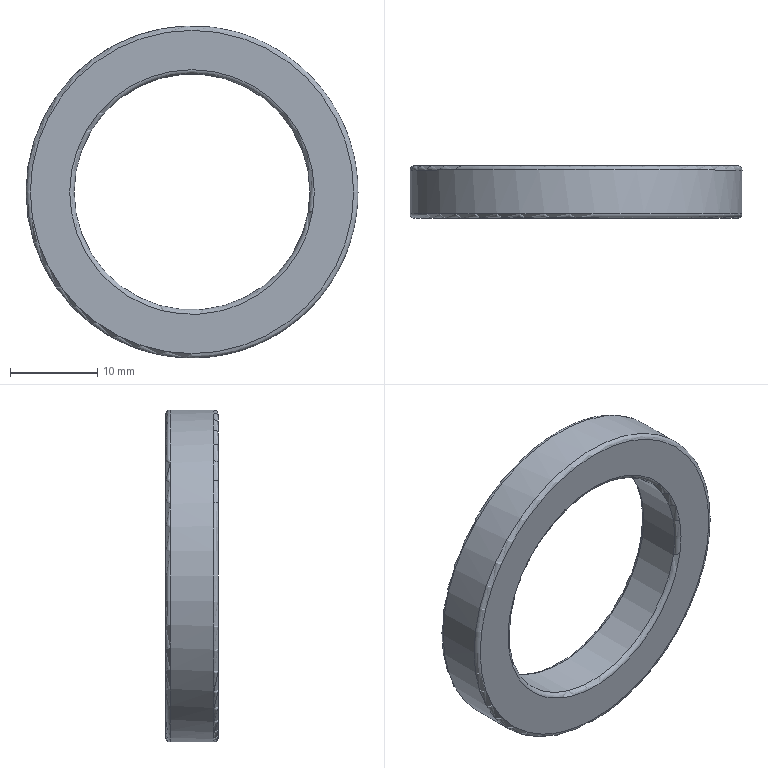Part | STEP file | BK-20_id1226_x_t | 1 solid | 12 faces | box 38 x 6 x 38 mm | volume 1557 mm3 | plane 4 | cylinder 4 | torus 4 | commonest cylinder face diameters 27 x1 29 x1 36 x1 38 x1
STEP:
#1=CARTESIAN_POINT('',(0.,0.,0.));
#2=DIRECTION('',(0.,0.,1.));
#3=DIRECTION('',(1.,0.,0.));
#4=AXIS2_PLACEMENT_3D('',#1,#2,#3);
#5=CARTESIAN_POINT('',(-283.,543.936,-165.5));
#6=VERTEX_POINT('',#5);
#7=CARTESIAN_POINT('',(-268.5,543.936,-165.5));
#8=DIRECTION('',(0.,1.,0.));
#9=DIRECTION('',(-1.,0.,0.));
#10=AXIS2_PLACEMENT_3D('',#7,#8,#9);
#11=CIRCLE('',#10,14.5);
#12=CARTESIAN_POINT('',(-268.5,543.936,-147.5));
#13=DIRECTION('',(0.,-1.,0.));
#14=DIRECTION('',(1.,0.,0.));
#15=AXIS2_PLACEMENT_3D('',#12,#13,#14);
#16=PLANE('',#15);
#17=CARTESIAN_POINT('',(-14.5,-18.));
#18=CARTESIAN_POINT('',(-14.5,7.115));
#19=CARTESIAN_POINT('',(7.25,-5.443));
#20=CARTESIAN_POINT('',(29.,-18.));
#21=CARTESIAN_POINT('',(7.25,-30.557));
#22=CARTESIAN_POINT('',(-14.5,-43.115));
#23=CARTESIAN_POINT('',(-14.5,-18.));
#24=(BOUNDED_CURVE()B_SPLINE_CURVE(2,(#17,#18,#19,#20,#21,#22,#23),.UNSPECIFIED.,.T.,.F.)B_SPLINE_CURVE_WITH_KNOTS((1,2,2,2,2,1),(-2.094,0.,2.094,4.189,6.283,8.378),.UNSPECIFIED.)CURVE()GEOMETRIC_REPRESENTATION_ITEM()RATIONAL_B_SPLINE_CURVE((1.,0.5,1.,0.5,1.,0.5,1.))REPRESENTATION_ITEM(''));
#25=(GEOMETRIC_REPRESENTATION_CONTEXT(2)PARAMETRIC_REPRESENTATION_CONTEXT()REPRESENTATION_CONTEXT('',''));
#26=DEFINITIONAL_REPRESENTATION('',(#24),#25);
#27=PCURVE('',#16,#26);
#28=CARTESIAN_POINT('',(-268.5,569.59,-165.5));
#29=DIRECTION('',(0.,1.,0.));
#30=DIRECTION('',(-1.,0.,0.));
#31=AXIS2_PLACEMENT_3D('',#28,#29,#30);
#32=CYLINDRICAL_SURFACE('',#31,14.5);
#33=CARTESIAN_POINT('',(0.,-25.654));
#34=DIRECTION('',(1.,0.));
#35=VECTOR('',#34,1.);
#36=LINE('',#33,#35);
#37=(GEOMETRIC_REPRESENTATION_CONTEXT(2)PARAMETRIC_REPRESENTATION_CONTEXT()REPRESENTATION_CONTEXT('',''));
#38=DEFINITIONAL_REPRESENTATION('',(#36),#37);
#39=PCURVE('',#32,#38);
#40=SURFACE_CURVE('',#11,(#27,#39),.PCURVE_S1.);
#41=EDGE_CURVE('',#6,#6,#40,.T.);
#42=ORIENTED_EDGE('',*,*,#41,.F.);
#43=EDGE_LOOP('',(#42));
#44=FACE_BOUND('',#43,.T.);
#45=CARTESIAN_POINT('',(-286.5,543.936,-165.5));
#46=VERTEX_POINT('',#45);
#47=CARTESIAN_POINT('',(-268.5,543.936,-165.5));
#48=DIRECTION('',(0.,1.,0.));
#49=DIRECTION('',(-1.,0.,0.));
#50=AXIS2_PLACEMENT_3D('',#47,#48,#49);
#51=CIRCLE('',#50,18.);
#52=CARTESIAN_POINT('',(-18.,-18.));
#53=CARTESIAN_POINT('',(-18.,13.177));
#54=CARTESIAN_POINT('',(9.,-2.412));
#55=CARTESIAN_POINT('',(36.,-18.));
#56=CARTESIAN_POINT('',(9.,-33.588));
#57=CARTESIAN_POINT('',(-18.,-49.177));
#58=CARTESIAN_POINT('',(-18.,-18.));
#59=(BOUNDED_CURVE()B_SPLINE_CURVE(2,(#52,#53,#54,#55,#56,#57,#58),.UNSPECIFIED.,.T.,.F.)B_SPLINE_CURVE_WITH_KNOTS((1,2,2,2,2,1),(-2.094,0.,2.094,4.189,6.283,8.378),.UNSPECIFIED.)CURVE()GEOMETRIC_REPRESENTATION_ITEM()RATIONAL_B_SPLINE_CURVE((1.,0.5,1.,0.5,1.,0.5,1.))REPRESENTATION_ITEM(''));
#60=(GEOMETRIC_REPRESENTATION_CONTEXT(2)PARAMETRIC_REPRESENTATION_CONTEXT()REPRESENTATION_CONTEXT('',''));
#61=DEFINITIONAL_REPRESENTATION('',(#59),#60);
#62=PCURVE('',#16,#61);
#63=CARTESIAN_POINT('',(-268.5,569.59,-165.5));
#64=DIRECTION('',(0.,1.,0.));
#65=DIRECTION('',(-1.,0.,0.));
#66=AXIS2_PLACEMENT_3D('',#63,#64,#65);
#67=CYLINDRICAL_SURFACE('',#66,18.);
#68=CARTESIAN_POINT('',(0.,-25.654));
#69=DIRECTION('',(1.,0.));
#70=VECTOR('',#69,1.);
#71=LINE('',#68,#70);
#72=(GEOMETRIC_REPRESENTATION_CONTEXT(2)PARAMETRIC_REPRESENTATION_CONTEXT()REPRESENTATION_CONTEXT('',''));
#73=DEFINITIONAL_REPRESENTATION('',(#71),#72);
#74=PCURVE('',#67,#73);
#75=SURFACE_CURVE('',#51,(#62,#74),.PCURVE_S1.);
#76=EDGE_CURVE('',#46,#46,#75,.T.);
#77=ORIENTED_EDGE('',*,*,#76,.T.);
#78=EDGE_LOOP('',(#77));
#79=FACE_BOUND('',#78,.T.);
#80=ADVANCED_FACE('',(#44,#79),#16,.F.);
#81=ORIENTED_EDGE('',*,*,#76,.T.);
#82=CARTESIAN_POINT('',(-286.5,548.936,-165.5));
#83=VERTEX_POINT('',#82);
#84=CARTESIAN_POINT('',(-286.5,543.936,-165.5));
#85=CARTESIAN_POINT('',(-286.5,548.936,-165.5));
#86=B_SPLINE_CURVE_WITH_KNOTS('',1,(#84,#85),.UNSPECIFIED.,.F.,.F.,(2,2),(-25.654,-20.654),.PIECEWISE_BEZIER_KNOTS.);
#87=CARTESIAN_POINT('',(6.283,0.));
#88=DIRECTION('',(0.,1.));
#89=VECTOR('',#88,1.);
#90=LINE('',#87,#89);
#91=(GEOMETRIC_REPRESENTATION_CONTEXT(2)PARAMETRIC_REPRESENTATION_CONTEXT()REPRESENTATION_CONTEXT('',''));
#92=DEFINITIONAL_REPRESENTATION('',(#90),#91);
#93=PCURVE('',#67,#92);
#94=CARTESIAN_POINT('',(0.,0.));
#95=DIRECTION('',(0.,1.));
#96=VECTOR('',#95,1.);
#97=LINE('',#94,#96);
#98=(GEOMETRIC_REPRESENTATION_CONTEXT(2)PARAMETRIC_REPRESENTATION_CONTEXT()REPRESENTATION_CONTEXT('',''));
#99=DEFINITIONAL_REPRESENTATION('',(#97),#98);
#100=PCURVE('',#67,#99);
#101=SEAM_CURVE('',#86,(#93,#100),.PCURVE_S1.);
#102=EDGE_CURVE('',#46,#83,#101,.T.);
#103=ORIENTED_EDGE('',*,*,#102,.T.);
#104=CARTESIAN_POINT('',(-268.5,548.936,-165.5));
#105=DIRECTION('',(0.,1.,0.));
#106=DIRECTION('',(-1.,0.,0.));
#107=AXIS2_PLACEMENT_3D('',#104,#105,#106);
#108=CIRCLE('',#107,18.);
#109=CARTESIAN_POINT('',(0.,-20.654));
#110=DIRECTION('',(1.,0.));
#111=VECTOR('',#110,1.);
#112=LINE('',#109,#111);
#113=(GEOMETRIC_REPRESENTATION_CONTEXT(2)PARAMETRIC_REPRESENTATION_CONTEXT()REPRESENTATION_CONTEXT('',''));
#114=DEFINITIONAL_REPRESENTATION('',(#112),#113);
#115=PCURVE('',#67,#114);
#116=CARTESIAN_POINT('',(-268.5,548.936,-146.5));
#117=DIRECTION('',(0.,-1.,0.));
#118=DIRECTION('',(1.,0.,0.));
#119=AXIS2_PLACEMENT_3D('',#116,#117,#118);
#120=PLANE('',#119);
#121=CARTESIAN_POINT('',(-18.,-19.));
#122=CARTESIAN_POINT('',(-18.,12.177));
#123=CARTESIAN_POINT('',(9.,-3.412));
#124=CARTESIAN_POINT('',(36.,-19.));
#125=CARTESIAN_POINT('',(9.,-34.588));
#126=CARTESIAN_POINT('',(-18.,-50.177));
#127=CARTESIAN_POINT('',(-18.,-19.));
#128=(BOUNDED_CURVE()B_SPLINE_CURVE(2,(#121,#122,#123,#124,#125,#126,#127),.UNSPECIFIED.,.T.,.F.)B_SPLINE_CURVE_WITH_KNOTS((1,2,2,2,2,1),(-2.094,0.,2.094,4.189,6.283,8.378),.UNSPECIFIED.)CURVE()GEOMETRIC_REPRESENTATION_ITEM()RATIONAL_B_SPLINE_CURVE((1.,0.5,1.,0.5,1.,0.5,1.))REPRESENTATION_ITEM(''));
#129=(GEOMETRIC_REPRESENTATION_CONTEXT(2)PARAMETRIC_REPRESENTATION_CONTEXT()REPRESENTATION_CONTEXT('',''));
#130=DEFINITIONAL_REPRESENTATION('',(#128),#129);
#131=PCURVE('',#120,#130);
#132=SURFACE_CURVE('',#108,(#115,#131),.PCURVE_S1.);
#133=EDGE_CURVE('',#83,#83,#132,.T.);
#134=ORIENTED_EDGE('',*,*,#133,.F.);
#135=ORIENTED_EDGE('',*,*,#102,.F.);
#136=EDGE_LOOP('',(#81,#103,#134,#135));
#137=FACE_BOUND('',#136,.F.);
#138=ADVANCED_FACE('',(#137),#67,.F.);
#139=ORIENTED_EDGE('',*,*,#41,.T.);
#140=CARTESIAN_POINT('',(-283.,548.936,-165.5));
#141=VERTEX_POINT('',#140);
#142=CARTESIAN_POINT('',(-283.,543.936,-165.5));
#143=CARTESIAN_POINT('',(-283.,548.936,-165.5));
#144=B_SPLINE_CURVE_WITH_KNOTS('',1,(#142,#143),.UNSPECIFIED.,.F.,.F.,(2,2),(-25.654,-20.654),.PIECEWISE_BEZIER_KNOTS.);
#145=CARTESIAN_POINT('',(6.283,0.));
#146=DIRECTION('',(0.,1.));
#147=VECTOR('',#146,1.);
#148=LINE('',#145,#147);
#149=(GEOMETRIC_REPRESENTATION_CONTEXT(2)PARAMETRIC_REPRESENTATION_CONTEXT()REPRESENTATION_CONTEXT('',''));
#150=DEFINITIONAL_REPRESENTATION('',(#148),#149);
#151=PCURVE('',#32,#150);
#152=CARTESIAN_POINT('',(0.,0.));
#153=DIRECTION('',(0.,1.));
#154=VECTOR('',#153,1.);
#155=LINE('',#152,#154);
#156=(GEOMETRIC_REPRESENTATION_CONTEXT(2)PARAMETRIC_REPRESENTATION_CONTEXT()REPRESENTATION_CONTEXT('',''));
#157=DEFINITIONAL_REPRESENTATION('',(#155),#156);
#158=PCURVE('',#32,#157);
#159=SEAM_CURVE('',#144,(#151,#158),.PCURVE_S1.);
#160=EDGE_CURVE('',#6,#141,#159,.T.);
#161=ORIENTED_EDGE('',*,*,#160,.T.);
#162=CARTESIAN_POINT('',(-268.5,548.936,-165.5));
#163=DIRECTION('',(0.,-1.,0.));
#164=DIRECTION('',(-1.,0.,0.));
#165=AXIS2_PLACEMENT_3D('',#162,#163,#164);
#166=CIRCLE('',#165,14.5);
#167=CARTESIAN_POINT('',(6.283,-20.654));
#168=DIRECTION('',(-1.,0.));
#169=VECTOR('',#168,1.);
#170=LINE('',#167,#169);
#171=(GEOMETRIC_REPRESENTATION_CONTEXT(2)PARAMETRIC_REPRESENTATION_CONTEXT()REPRESENTATION_CONTEXT('',''));
#172=DEFINITIONAL_REPRESENTATION('',(#170),#171);
#173=PCURVE('',#32,#172);
#174=CARTESIAN_POINT('',(-268.5,548.936,-151.));
#175=DIRECTION('',(0.,-1.,0.));
#176=DIRECTION('',(1.,0.,0.));
#177=AXIS2_PLACEMENT_3D('',#174,#175,#176);
#178=PLANE('',#177);
#179=CARTESIAN_POINT('',(0.,-14.5));
#180=DIRECTION('',(-1.,0.));
#181=AXIS2_PLACEMENT_2D('',#179,#180);
#182=CIRCLE('',#181,14.5);
#183=(GEOMETRIC_REPRESENTATION_CONTEXT(2)PARAMETRIC_REPRESENTATION_CONTEXT()REPRESENTATION_CONTEXT('',''));
#184=DEFINITIONAL_REPRESENTATION('',(#182),#183);
#185=PCURVE('',#178,#184);
#186=SURFACE_CURVE('',#166,(#173,#185),.PCURVE_S1.);
#187=EDGE_CURVE('',#141,#141,#186,.T.);
#188=ORIENTED_EDGE('',*,*,#187,.T.);
#189=ORIENTED_EDGE('',*,*,#160,.F.);
#190=EDGE_LOOP('',(#139,#161,#188,#189));
#191=FACE_BOUND('',#190,.T.);
#192=ADVANCED_FACE('',(#191),#32,.T.);
#193=CARTESIAN_POINT('',(-250.,548.936,-165.5));
#194=VERTEX_POINT('',#193);
#195=CARTESIAN_POINT('',(-268.5,548.936,-165.5));
#196=DIRECTION('',(0.,-1.,0.));
#197=DIRECTION('',(1.,0.,0.));
#198=AXIS2_PLACEMENT_3D('',#195,#196,#197);
#199=CIRCLE('',#198,18.5);
#200=CARTESIAN_POINT('',(0.,-19.));
#201=DIRECTION('',(1.,0.));
#202=AXIS2_PLACEMENT_2D('',#200,#201);
#203=CIRCLE('',#202,18.5);
#204=(GEOMETRIC_REPRESENTATION_CONTEXT(2)PARAMETRIC_REPRESENTATION_CONTEXT()REPRESENTATION_CONTEXT('',''));
#205=DEFINITIONAL_REPRESENTATION('',(#203),#204);
#206=PCURVE('',#120,#205);
#207=CARTESIAN_POINT('',(-268.5,548.436,-165.5));
#208=DIRECTION('',(0.,-1.,0.));
#209=DIRECTION('',(1.,0.,0.));
#210=AXIS2_PLACEMENT_3D('',#207,#208,#209);
#211=TOROIDAL_SURFACE('',#210,18.5,0.5);
#212=CARTESIAN_POINT('',(0.,4.712));
#213=DIRECTION('',(1.,0.));
#214=VECTOR('',#213,1.);
#215=LINE('',#212,#214);
#216=(GEOMETRIC_REPRESENTATION_CONTEXT(2)PARAMETRIC_REPRESENTATION_CONTEXT()REPRESENTATION_CONTEXT('',''));
#217=DEFINITIONAL_REPRESENTATION('',(#215),#216);
#218=PCURVE('',#211,#217);
#219=SURFACE_CURVE('',#199,(#206,#218),.PCURVE_S1.);
#220=EDGE_CURVE('',#194,#194,#219,.T.);
#221=ORIENTED_EDGE('',*,*,#220,.F.);
#222=EDGE_LOOP('',(#221));
#223=FACE_BOUND('',#222,.T.);
#224=ORIENTED_EDGE('',*,*,#133,.F.);
#225=EDGE_LOOP('',(#224));
#226=FACE_BOUND('',#225,.T.);
#227=ADVANCED_FACE('',(#223,#226),#120,.F.);
#228=CARTESIAN_POINT('',(-254.5,548.936,-165.5));
#229=VERTEX_POINT('',#228);
#230=CARTESIAN_POINT('',(-268.5,548.936,-165.5));
#231=DIRECTION('',(0.,1.,0.));
#232=DIRECTION('',(1.,0.,0.));
#233=AXIS2_PLACEMENT_3D('',#230,#231,#232);
#234=CIRCLE('',#233,14.);
#235=CARTESIAN_POINT('',(14.,-14.5));
#236=CARTESIAN_POINT('',(14.,-38.749));
#237=CARTESIAN_POINT('',(-7.,-26.624));
#238=CARTESIAN_POINT('',(-28.,-14.5));
#239=CARTESIAN_POINT('',(-7.,-2.376));
#240=CARTESIAN_POINT('',(14.,9.749));
#241=CARTESIAN_POINT('',(14.,-14.5));
#242=(BOUNDED_CURVE()B_SPLINE_CURVE(2,(#235,#236,#237,#238,#239,#240,#241),.UNSPECIFIED.,.T.,.F.)B_SPLINE_CURVE_WITH_KNOTS((1,2,2,2,2,1),(-2.094,0.,2.094,4.189,6.283,8.378),.UNSPECIFIED.)CURVE()GEOMETRIC_REPRESENTATION_ITEM()RATIONAL_B_SPLINE_CURVE((1.,0.5,1.,0.5,1.,0.5,1.))REPRESENTATION_ITEM(''));
#243=(GEOMETRIC_REPRESENTATION_CONTEXT(2)PARAMETRIC_REPRESENTATION_CONTEXT()REPRESENTATION_CONTEXT('',''));
#244=DEFINITIONAL_REPRESENTATION('',(#242),#243);
#245=PCURVE('',#178,#244);
#246=CARTESIAN_POINT('',(-268.5,548.436,-165.5));
#247=DIRECTION('',(0.,-1.,0.));
#248=DIRECTION('',(1.,0.,0.));
#249=AXIS2_PLACEMENT_3D('',#246,#247,#248);
#250=TOROIDAL_SURFACE('',#249,14.,0.5);
#251=CARTESIAN_POINT('',(6.283,4.712));
#252=DIRECTION('',(-1.,0.));
#253=VECTOR('',#252,1.);
#254=LINE('',#251,#253);
#255=(GEOMETRIC_REPRESENTATION_CONTEXT(2)PARAMETRIC_REPRESENTATION_CONTEXT()REPRESENTATION_CONTEXT('',''));
#256=DEFINITIONAL_REPRESENTATION('',(#254),#255);
#257=PCURVE('',#250,#256);
#258=SURFACE_CURVE('',#234,(#245,#257),.PCURVE_S1.);
#259=EDGE_CURVE('',#229,#229,#258,.T.);
#260=ORIENTED_EDGE('',*,*,#259,.F.);
#261=EDGE_LOOP('',(#260));
#262=FACE_BOUND('',#261,.T.);
#263=ORIENTED_EDGE('',*,*,#187,.F.);
#264=EDGE_LOOP('',(#263));
#265=FACE_BOUND('',#264,.T.);
#266=ADVANCED_FACE('',(#262,#265),#178,.F.);
#267=CARTESIAN_POINT('',(-249.5,548.436,-165.5));
#268=VERTEX_POINT('',#267);
#269=CARTESIAN_POINT('',(-287.5,548.436,-165.5));
#270=VERTEX_POINT('',#269);
#271=CARTESIAN_POINT('',(-268.5,548.436,-165.5));
#272=DIRECTION('',(0.,-1.,0.));
#273=DIRECTION('',(-1.,0.,0.));
#274=AXIS2_PLACEMENT_3D('',#271,#272,#273);
#275=CIRCLE('',#274,19.);
#276=CARTESIAN_POINT('',(-3.142,6.283));
#277=DIRECTION('',(1.,0.));
#278=VECTOR('',#277,1.);
#279=LINE('',#276,#278);
#280=(GEOMETRIC_REPRESENTATION_CONTEXT(2)PARAMETRIC_REPRESENTATION_CONTEXT()REPRESENTATION_CONTEXT('',''));
#281=DEFINITIONAL_REPRESENTATION('',(#279),#280);
#282=PCURVE('',#211,#281);
#283=CARTESIAN_POINT('',(-268.5,569.59,-165.5));
#284=DIRECTION('',(0.,1.,0.));
#285=DIRECTION('',(-1.,0.,0.));
#286=AXIS2_PLACEMENT_3D('',#283,#284,#285);
#287=CYLINDRICAL_SURFACE('',#286,19.);
#288=CARTESIAN_POINT('',(6.283,-21.154));
#289=DIRECTION('',(-1.,0.));
#290=VECTOR('',#289,1.);
#291=LINE('',#288,#290);
#292=(GEOMETRIC_REPRESENTATION_CONTEXT(2)PARAMETRIC_REPRESENTATION_CONTEXT()REPRESENTATION_CONTEXT('',''));
#293=DEFINITIONAL_REPRESENTATION('',(#291),#292);
#294=PCURVE('',#287,#293);
#295=SURFACE_CURVE('',#275,(#282,#294),.PCURVE_S1.);
#296=EDGE_CURVE('',#268,#270,#295,.T.);
#297=ORIENTED_EDGE('',*,*,#296,.F.);
#298=CARTESIAN_POINT('',(-250.,548.936,-165.5));
#299=CARTESIAN_POINT('',(-249.866,548.936,-165.5));
#300=CARTESIAN_POINT('',(-249.736,548.893,-165.5));
#301=CARTESIAN_POINT('',(-249.624,548.812,-165.5));
#302=CARTESIAN_POINT('',(-249.543,548.699,-165.5));
#303=CARTESIAN_POINT('',(-249.5,548.569,-165.5));
#304=CARTESIAN_POINT('',(-249.5,548.436,-165.5));
#305=(BOUNDED_CURVE()B_SPLINE_CURVE(6,(#298,#299,#300,#301,#302,#303,#304),.UNSPECIFIED.,.F.,.F.)B_SPLINE_CURVE_WITH_KNOTS((7,7),(-1.571,0.),.PIECEWISE_BEZIER_KNOTS.)CURVE()GEOMETRIC_REPRESENTATION_ITEM()RATIONAL_B_SPLINE_CURVE((1.031,1.01,0.9979,0.994,0.9979,1.01,1.031))REPRESENTATION_ITEM(''));
#306=CARTESIAN_POINT('',(0.,6.283));
#307=DIRECTION('',(0.,1.));
#308=VECTOR('',#307,1.);
#309=LINE('',#306,#308);
#310=(GEOMETRIC_REPRESENTATION_CONTEXT(2)PARAMETRIC_REPRESENTATION_CONTEXT()REPRESENTATION_CONTEXT('',''));
#311=DEFINITIONAL_REPRESENTATION('',(#309),#310);
#312=PCURVE('',#211,#311);
#313=CARTESIAN_POINT('',(6.283,6.283));
#314=DIRECTION('',(0.,1.));
#315=VECTOR('',#314,1.);
#316=LINE('',#313,#315);
#317=(GEOMETRIC_REPRESENTATION_CONTEXT(2)PARAMETRIC_REPRESENTATION_CONTEXT()REPRESENTATION_CONTEXT('',''));
#318=DEFINITIONAL_REPRESENTATION('',(#316),#317);
#319=PCURVE('',#211,#318);
#320=SEAM_CURVE('',#305,(#312,#319),.PCURVE_S1.);
#321=EDGE_CURVE('',#194,#268,#320,.T.);
#322=ORIENTED_EDGE('',*,*,#321,.F.);
#323=ORIENTED_EDGE('',*,*,#220,.T.);
#324=ORIENTED_EDGE('',*,*,#321,.T.);
#325=CARTESIAN_POINT('',(-268.5,548.436,-165.5));
#326=DIRECTION('',(0.,-1.,0.));
#327=DIRECTION('',(-1.,0.,0.));
#328=AXIS2_PLACEMENT_3D('',#325,#326,#327);
#329=CIRCLE('',#328,19.);
#330=CARTESIAN_POINT('',(3.142,6.283));
#331=DIRECTION('',(1.,0.));
#332=VECTOR('',#331,1.);
#333=LINE('',#330,#332);
#334=(GEOMETRIC_REPRESENTATION_CONTEXT(2)PARAMETRIC_REPRESENTATION_CONTEXT()REPRESENTATION_CONTEXT('',''));
#335=DEFINITIONAL_REPRESENTATION('',(#333),#334);
#336=PCURVE('',#211,#335);
#337=CARTESIAN_POINT('',(6.283,-21.154));
#338=DIRECTION('',(-1.,0.));
#339=VECTOR('',#338,1.);
#340=LINE('',#337,#339);
#341=(GEOMETRIC_REPRESENTATION_CONTEXT(2)PARAMETRIC_REPRESENTATION_CONTEXT()REPRESENTATION_CONTEXT('',''));
#342=DEFINITIONAL_REPRESENTATION('',(#340),#341);
#343=PCURVE('',#287,#342);
#344=SURFACE_CURVE('',#329,(#336,#343),.PCURVE_S1.);
#345=EDGE_CURVE('',#270,#268,#344,.T.);
#346=ORIENTED_EDGE('',*,*,#345,.F.);
#347=EDGE_LOOP('',(#297,#322,#323,#324,#346));
#348=FACE_BOUND('',#347,.T.);
#349=ADVANCED_FACE('',(#348),#211,.T.);
#350=CARTESIAN_POINT('',(-282.,548.436,-165.5));
#351=VERTEX_POINT('',#350);
#352=CARTESIAN_POINT('',(-255.,548.436,-165.5));
#353=VERTEX_POINT('',#352);
#354=CARTESIAN_POINT('',(-268.5,548.436,-165.5));
#355=DIRECTION('',(0.,-1.,0.));
#356=DIRECTION('',(-1.,0.,0.));
#357=AXIS2_PLACEMENT_3D('',#354,#355,#356);
#358=CIRCLE('',#357,13.5);
#359=CARTESIAN_POINT('',(3.142,3.142));
#360=DIRECTION('',(1.,0.));
#361=VECTOR('',#360,1.);
#362=LINE('',#359,#361);
#363=(GEOMETRIC_REPRESENTATION_CONTEXT(2)PARAMETRIC_REPRESENTATION_CONTEXT()REPRESENTATION_CONTEXT('',''));
#364=DEFINITIONAL_REPRESENTATION('',(#362),#363);
#365=PCURVE('',#250,#364);
#366=CARTESIAN_POINT('',(-268.5,569.59,-165.5));
#367=DIRECTION('',(0.,1.,0.));
#368=DIRECTION('',(-1.,0.,0.));
#369=AXIS2_PLACEMENT_3D('',#366,#367,#368);
#370=CYLINDRICAL_SURFACE('',#369,13.5);
#371=CARTESIAN_POINT('',(6.283,-21.154));
#372=DIRECTION('',(-1.,0.));
#373=VECTOR('',#372,1.);
#374=LINE('',#371,#373);
#375=(GEOMETRIC_REPRESENTATION_CONTEXT(2)PARAMETRIC_REPRESENTATION_CONTEXT()REPRESENTATION_CONTEXT('',''));
#376=DEFINITIONAL_REPRESENTATION('',(#374),#375);
#377=PCURVE('',#370,#376);
#378=SURFACE_CURVE('',#358,(#365,#377),.PCURVE_S1.);
#379=EDGE_CURVE('',#351,#353,#378,.T.);
#380=ORIENTED_EDGE('',*,*,#379,.T.);
#381=CARTESIAN_POINT('',(-255.,548.436,-165.5));
#382=CARTESIAN_POINT('',(-255.,548.569,-165.5));
#383=CARTESIAN_POINT('',(-254.957,548.699,-165.5));
#384=CARTESIAN_POINT('',(-254.876,548.812,-165.5));
#385=CARTESIAN_POINT('',(-254.764,548.893,-165.5));
#386=CARTESIAN_POINT('',(-254.634,548.936,-165.5));
#387=CARTESIAN_POINT('',(-254.5,548.936,-165.5));
#388=(BOUNDED_CURVE()B_SPLINE_CURVE(6,(#381,#382,#383,#384,#385,#386,#387),.UNSPECIFIED.,.F.,.F.)B_SPLINE_CURVE_WITH_KNOTS((7,7),(3.142,4.712),.PIECEWISE_BEZIER_KNOTS.)CURVE()GEOMETRIC_REPRESENTATION_ITEM()RATIONAL_B_SPLINE_CURVE((1.031,1.01,0.9979,0.994,0.9979,1.01,1.031))REPRESENTATION_ITEM(''));
#389=CARTESIAN_POINT('',(6.283,0.));
#390=DIRECTION('',(0.,1.));
#391=VECTOR('',#390,1.);
#392=LINE('',#389,#391);
#393=(GEOMETRIC_REPRESENTATION_CONTEXT(2)PARAMETRIC_REPRESENTATION_CONTEXT()REPRESENTATION_CONTEXT('',''));
#394=DEFINITIONAL_REPRESENTATION('',(#392),#393);
#395=PCURVE('',#250,#394);
#396=CARTESIAN_POINT('',(0.,0.));
#397=DIRECTION('',(0.,1.));
#398=VECTOR('',#397,1.);
#399=LINE('',#396,#398);
#400=(GEOMETRIC_REPRESENTATION_CONTEXT(2)PARAMETRIC_REPRESENTATION_CONTEXT()REPRESENTATION_CONTEXT('',''));
#401=DEFINITIONAL_REPRESENTATION('',(#399),#400);
#402=PCURVE('',#250,#401);
#403=SEAM_CURVE('',#388,(#395,#402),.PCURVE_S1.);
#404=EDGE_CURVE('',#353,#229,#403,.T.);
#405=ORIENTED_EDGE('',*,*,#404,.T.);
#406=ORIENTED_EDGE('',*,*,#259,.T.);
#407=ORIENTED_EDGE('',*,*,#404,.F.);
#408=CARTESIAN_POINT('',(-268.5,548.436,-165.5));
#409=DIRECTION('',(0.,-1.,0.));
#410=DIRECTION('',(-1.,0.,0.));
#411=AXIS2_PLACEMENT_3D('',#408,#409,#410);
#412=CIRCLE('',#411,13.5);
#413=CARTESIAN_POINT('',(-3.142,3.142));
#414=DIRECTION('',(1.,0.));
#415=VECTOR('',#414,1.);
#416=LINE('',#413,#415);
#417=(GEOMETRIC_REPRESENTATION_CONTEXT(2)PARAMETRIC_REPRESENTATION_CONTEXT()REPRESENTATION_CONTEXT('',''));
#418=DEFINITIONAL_REPRESENTATION('',(#416),#417);
#419=PCURVE('',#250,#418);
#420=CARTESIAN_POINT('',(12.566,-21.154));
#421=DIRECTION('',(-1.,0.));
#422=VECTOR('',#421,1.);
#423=LINE('',#420,#422);
#424=(GEOMETRIC_REPRESENTATION_CONTEXT(2)PARAMETRIC_REPRESENTATION_CONTEXT()REPRESENTATION_CONTEXT('',''));
#425=DEFINITIONAL_REPRESENTATION('',(#423),#424);
#426=PCURVE('',#370,#425);
#427=SURFACE_CURVE('',#412,(#419,#426),.PCURVE_S1.);
#428=EDGE_CURVE('',#353,#351,#427,.T.);
#429=ORIENTED_EDGE('',*,*,#428,.T.);
#430=EDGE_LOOP('',(#380,#405,#406,#407,#429));
#431=FACE_BOUND('',#430,.T.);
#432=ADVANCED_FACE('',(#431),#250,.T.);
#433=ORIENTED_EDGE('',*,*,#345,.T.);
#434=ORIENTED_EDGE('',*,*,#296,.T.);
#435=CARTESIAN_POINT('',(-287.5,543.436,-165.5));
#436=VERTEX_POINT('',#435);
#437=CARTESIAN_POINT('',(-287.5,543.436,-165.5));
#438=CARTESIAN_POINT('',(-287.5,548.436,-165.5));
#439=B_SPLINE_CURVE_WITH_KNOTS('',1,(#437,#438),.UNSPECIFIED.,.F.,.F.,(2,2),(-26.154,-21.154),.PIECEWISE_BEZIER_KNOTS.);
#440=CARTESIAN_POINT('',(0.,0.));
#441=DIRECTION('',(0.,1.));
#442=VECTOR('',#441,1.);
#443=LINE('',#440,#442);
#444=(GEOMETRIC_REPRESENTATION_CONTEXT(2)PARAMETRIC_REPRESENTATION_CONTEXT()REPRESENTATION_CONTEXT('',''));
#445=DEFINITIONAL_REPRESENTATION('',(#443),#444);
#446=PCURVE('',#287,#445);
#447=CARTESIAN_POINT('',(6.283,0.));
#448=DIRECTION('',(0.,1.));
#449=VECTOR('',#448,1.);
#450=LINE('',#447,#449);
#451=(GEOMETRIC_REPRESENTATION_CONTEXT(2)PARAMETRIC_REPRESENTATION_CONTEXT()REPRESENTATION_CONTEXT('',''));
#452=DEFINITIONAL_REPRESENTATION('',(#450),#451);
#453=PCURVE('',#287,#452);
#454=SEAM_CURVE('',#439,(#446,#453),.PCURVE_S1.);
#455=EDGE_CURVE('',#436,#270,#454,.T.);
#456=ORIENTED_EDGE('',*,*,#455,.F.);
#457=CARTESIAN_POINT('',(-268.5,543.436,-165.5));
#458=DIRECTION('',(0.,-1.,0.));
#459=DIRECTION('',(-1.,0.,0.));
#460=AXIS2_PLACEMENT_3D('',#457,#458,#459);
#461=CIRCLE('',#460,19.);
#462=CARTESIAN_POINT('',(6.283,-26.154));
#463=DIRECTION('',(-1.,0.));
#464=VECTOR('',#463,1.);
#465=LINE('',#462,#464);
#466=(GEOMETRIC_REPRESENTATION_CONTEXT(2)PARAMETRIC_REPRESENTATION_CONTEXT()REPRESENTATION_CONTEXT('',''));
#467=DEFINITIONAL_REPRESENTATION('',(#465),#466);
#468=PCURVE('',#287,#467);
#469=CARTESIAN_POINT('',(-268.5,543.436,-165.5));
#470=DIRECTION('',(0.,1.,0.));
#471=DIRECTION('',(-1.,0.,0.));
#472=AXIS2_PLACEMENT_3D('',#469,#470,#471);
#473=TOROIDAL_SURFACE('',#472,18.5,0.5);
#474=CARTESIAN_POINT('',(6.283,6.283));
#475=DIRECTION('',(-1.,0.));
#476=VECTOR('',#475,1.);
#477=LINE('',#474,#476);
#478=(GEOMETRIC_REPRESENTATION_CONTEXT(2)PARAMETRIC_REPRESENTATION_CONTEXT()REPRESENTATION_CONTEXT('',''));
#479=DEFINITIONAL_REPRESENTATION('',(#477),#478);
#480=PCURVE('',#473,#479);
#481=SURFACE_CURVE('',#461,(#468,#480),.PCURVE_S1.);
#482=EDGE_CURVE('',#436,#436,#481,.T.);
#483=ORIENTED_EDGE('',*,*,#482,.F.);
#484=ORIENTED_EDGE('',*,*,#455,.T.);
#485=EDGE_LOOP('',(#433,#434,#456,#483,#484));
#486=FACE_BOUND('',#485,.T.);
#487=ADVANCED_FACE('',(#486),#287,.T.);
#488=ORIENTED_EDGE('',*,*,#428,.T.);
#489=ORIENTED_EDGE('',*,*,#379,.T.);
#490=CARTESIAN_POINT('',(-255.,543.436,-165.5));
#491=VERTEX_POINT('',#490);
#492=CARTESIAN_POINT('',(-255.,543.436,-165.5));
#493=CARTESIAN_POINT('',(-255.,548.436,-165.5));
#494=B_SPLINE_CURVE_WITH_KNOTS('',1,(#492,#493),.UNSPECIFIED.,.F.,.F.,(2,2),(-26.154,-21.154),.PIECEWISE_BEZIER_KNOTS.);
#495=CARTESIAN_POINT('',(3.142,0.));
#496=DIRECTION('',(0.,1.));
#497=VECTOR('',#496,1.);
#498=LINE('',#495,#497);
#499=(GEOMETRIC_REPRESENTATION_CONTEXT(2)PARAMETRIC_REPRESENTATION_CONTEXT()REPRESENTATION_CONTEXT('',''));
#500=DEFINITIONAL_REPRESENTATION('',(#498),#499);
#501=PCURVE('',#370,#500);
#502=CARTESIAN_POINT('',(9.425,0.));
#503=DIRECTION('',(0.,1.));
#504=VECTOR('',#503,1.);
#505=LINE('',#502,#504);
#506=(GEOMETRIC_REPRESENTATION_CONTEXT(2)PARAMETRIC_REPRESENTATION_CONTEXT()REPRESENTATION_CONTEXT('',''));
#507=DEFINITIONAL_REPRESENTATION('',(#505),#506);
#508=PCURVE('',#370,#507);
#509=SEAM_CURVE('',#494,(#501,#508),.PCURVE_S1.);
#510=EDGE_CURVE('',#491,#353,#509,.T.);
#511=ORIENTED_EDGE('',*,*,#510,.F.);
#512=CARTESIAN_POINT('',(-268.5,543.436,-165.5));
#513=DIRECTION('',(0.,1.,0.));
#514=DIRECTION('',(1.,0.,0.));
#515=AXIS2_PLACEMENT_3D('',#512,#513,#514);
#516=CIRCLE('',#515,13.5);
#517=CARTESIAN_POINT('',(3.142,-26.154));
#518=DIRECTION('',(1.,0.));
#519=VECTOR('',#518,1.);
#520=LINE('',#517,#519);
#521=(GEOMETRIC_REPRESENTATION_CONTEXT(2)PARAMETRIC_REPRESENTATION_CONTEXT()REPRESENTATION_CONTEXT('',''));
#522=DEFINITIONAL_REPRESENTATION('',(#520),#521);
#523=PCURVE('',#370,#522);
#524=CARTESIAN_POINT('',(-268.5,543.436,-165.5));
#525=DIRECTION('',(0.,1.,0.));
#526=DIRECTION('',(0.,0.,-1.));
#527=AXIS2_PLACEMENT_3D('',#524,#525,#526);
#528=TOROIDAL_SURFACE('',#527,14.,0.5);
#529=CARTESIAN_POINT('',(4.712,3.142));
#530=DIRECTION('',(1.,0.));
#531=VECTOR('',#530,1.);
#532=LINE('',#529,#531);
#533=(GEOMETRIC_REPRESENTATION_CONTEXT(2)PARAMETRIC_REPRESENTATION_CONTEXT()REPRESENTATION_CONTEXT('',''));
#534=DEFINITIONAL_REPRESENTATION('',(#532),#533);
#535=PCURVE('',#528,#534);
#536=SURFACE_CURVE('',#516,(#523,#535),.PCURVE_S1.);
#537=EDGE_CURVE('',#491,#491,#536,.T.);
#538=ORIENTED_EDGE('',*,*,#537,.T.);
#539=ORIENTED_EDGE('',*,*,#510,.T.);
#540=EDGE_LOOP('',(#488,#489,#511,#538,#539));
#541=FACE_BOUND('',#540,.F.);
#542=ADVANCED_FACE('',(#541),#370,.F.);
#543=ORIENTED_EDGE('',*,*,#482,.T.);
#544=CARTESIAN_POINT('',(-287.,542.936,-165.5));
#545=VERTEX_POINT('',#544);
#546=CARTESIAN_POINT('',(-287.,542.936,-165.5));
#547=CARTESIAN_POINT('',(-287.134,542.936,-165.5));
#548=CARTESIAN_POINT('',(-287.264,542.978,-165.5));
#549=CARTESIAN_POINT('',(-287.376,543.06,-165.5));
#550=CARTESIAN_POINT('',(-287.457,543.172,-165.5));
#551=CARTESIAN_POINT('',(-287.5,543.302,-165.5));
#552=CARTESIAN_POINT('',(-287.5,543.436,-165.5));
#553=(BOUNDED_CURVE()B_SPLINE_CURVE(6,(#546,#547,#548,#549,#550,#551,#552),.UNSPECIFIED.,.F.,.F.)B_SPLINE_CURVE_WITH_KNOTS((7,7),(-1.571,0.),.PIECEWISE_BEZIER_KNOTS.)CURVE()GEOMETRIC_REPRESENTATION_ITEM()RATIONAL_B_SPLINE_CURVE((1.031,1.01,0.9979,0.994,0.9979,1.01,1.031))REPRESENTATION_ITEM(''));
#554=CARTESIAN_POINT('',(0.,6.283));
#555=DIRECTION('',(0.,1.));
#556=VECTOR('',#555,1.);
#557=LINE('',#554,#556);
#558=(GEOMETRIC_REPRESENTATION_CONTEXT(2)PARAMETRIC_REPRESENTATION_CONTEXT()REPRESENTATION_CONTEXT('',''));
#559=DEFINITIONAL_REPRESENTATION('',(#557),#558);
#560=PCURVE('',#473,#559);
#561=CARTESIAN_POINT('',(6.283,6.283));
#562=DIRECTION('',(0.,1.));
#563=VECTOR('',#562,1.);
#564=LINE('',#561,#563);
#565=(GEOMETRIC_REPRESENTATION_CONTEXT(2)PARAMETRIC_REPRESENTATION_CONTEXT()REPRESENTATION_CONTEXT('',''));
#566=DEFINITIONAL_REPRESENTATION('',(#564),#565);
#567=PCURVE('',#473,#566);
#568=SEAM_CURVE('',#553,(#560,#567),.PCURVE_S1.);
#569=EDGE_CURVE('',#545,#436,#568,.T.);
#570=ORIENTED_EDGE('',*,*,#569,.F.);
#571=CARTESIAN_POINT('',(-268.5,542.936,-165.5));
#572=DIRECTION('',(0.,1.,0.));
#573=DIRECTION('',(-1.,0.,0.));
#574=AXIS2_PLACEMENT_3D('',#571,#572,#573);
#575=CIRCLE('',#574,18.5);
#576=CARTESIAN_POINT('',(0.,4.712));
#577=DIRECTION('',(1.,0.));
#578=VECTOR('',#577,1.);
#579=LINE('',#576,#578);
#580=(GEOMETRIC_REPRESENTATION_CONTEXT(2)PARAMETRIC_REPRESENTATION_CONTEXT()REPRESENTATION_CONTEXT('',''));
#581=DEFINITIONAL_REPRESENTATION('',(#579),#580);
#582=PCURVE('',#473,#581);
#583=CARTESIAN_POINT('',(-268.5,542.936,-146.5));
#584=DIRECTION('',(0.,1.,0.));
#585=DIRECTION('',(-1.,0.,0.));
#586=AXIS2_PLACEMENT_3D('',#583,#584,#585);
#587=PLANE('',#586);
#588=CARTESIAN_POINT('',(0.,-19.));
#589=DIRECTION('',(1.,0.));
#590=AXIS2_PLACEMENT_2D('',#588,#589);
#591=CIRCLE('',#590,18.5);
#592=(GEOMETRIC_REPRESENTATION_CONTEXT(2)PARAMETRIC_REPRESENTATION_CONTEXT()REPRESENTATION_CONTEXT('',''));
#593=DEFINITIONAL_REPRESENTATION('',(#591),#592);
#594=PCURVE('',#587,#593);
#595=SURFACE_CURVE('',#575,(#582,#594),.PCURVE_S1.);
#596=EDGE_CURVE('',#545,#545,#595,.T.);
#597=ORIENTED_EDGE('',*,*,#596,.T.);
#598=ORIENTED_EDGE('',*,*,#569,.T.);
#599=EDGE_LOOP('',(#543,#570,#597,#598));
#600=FACE_BOUND('',#599,.T.);
#601=ADVANCED_FACE('',(#600),#473,.T.);
#602=ORIENTED_EDGE('',*,*,#537,.T.);
#603=CARTESIAN_POINT('',(-254.5,542.936,-165.5));
#604=VERTEX_POINT('',#603);
#605=CARTESIAN_POINT('',(-255.,543.436,-165.5));
#606=CARTESIAN_POINT('',(-255.,543.302,-165.5));
#607=CARTESIAN_POINT('',(-254.957,543.172,-165.5));
#608=CARTESIAN_POINT('',(-254.876,543.06,-165.5));
#609=CARTESIAN_POINT('',(-254.764,542.978,-165.5));
#610=CARTESIAN_POINT('',(-254.634,542.936,-165.5));
#611=CARTESIAN_POINT('',(-254.5,542.936,-165.5));
#612=(BOUNDED_CURVE()B_SPLINE_CURVE(6,(#605,#606,#607,#608,#609,#610,#611),.UNSPECIFIED.,.F.,.F.)B_SPLINE_CURVE_WITH_KNOTS((7,7),(3.142,4.712),.PIECEWISE_BEZIER_KNOTS.)CURVE()GEOMETRIC_REPRESENTATION_ITEM()RATIONAL_B_SPLINE_CURVE((1.031,1.01,0.9979,0.994,0.9979,1.01,1.031))REPRESENTATION_ITEM(''));
#613=CARTESIAN_POINT('',(10.996,0.));
#614=DIRECTION('',(0.,1.));
#615=VECTOR('',#614,1.);
#616=LINE('',#613,#615);
#617=(GEOMETRIC_REPRESENTATION_CONTEXT(2)PARAMETRIC_REPRESENTATION_CONTEXT()REPRESENTATION_CONTEXT('',''));
#618=DEFINITIONAL_REPRESENTATION('',(#616),#617);
#619=PCURVE('',#528,#618);
#620=CARTESIAN_POINT('',(4.712,0.));
#621=DIRECTION('',(0.,1.));
#622=VECTOR('',#621,1.);
#623=LINE('',#620,#622);
#624=(GEOMETRIC_REPRESENTATION_CONTEXT(2)PARAMETRIC_REPRESENTATION_CONTEXT()REPRESENTATION_CONTEXT('',''));
#625=DEFINITIONAL_REPRESENTATION('',(#623),#624);
#626=PCURVE('',#528,#625);
#627=SEAM_CURVE('',#612,(#619,#626),.PCURVE_S1.);
#628=EDGE_CURVE('',#491,#604,#627,.T.);
#629=ORIENTED_EDGE('',*,*,#628,.T.);
#630=CARTESIAN_POINT('',(-282.5,542.936,-165.5));
#631=VERTEX_POINT('',#630);
#632=CARTESIAN_POINT('',(-268.5,542.936,-165.5));
#633=DIRECTION('',(0.,-1.,0.));
#634=DIRECTION('',(0.,0.,-1.));
#635=AXIS2_PLACEMENT_3D('',#632,#633,#634);
#636=CIRCLE('',#635,14.);
#637=CARTESIAN_POINT('',(12.566,4.712));
#638=DIRECTION('',(-1.,0.));
#639=VECTOR('',#638,1.);
#640=LINE('',#637,#639);
#641=(GEOMETRIC_REPRESENTATION_CONTEXT(2)PARAMETRIC_REPRESENTATION_CONTEXT()REPRESENTATION_CONTEXT('',''));
#642=DEFINITIONAL_REPRESENTATION('',(#640),#641);
#643=PCURVE('',#528,#642);
#644=CARTESIAN_POINT('',(0.,-33.));
#645=CARTESIAN_POINT('',(-24.249,-33.));
#646=CARTESIAN_POINT('',(-12.124,-12.));
#647=CARTESIAN_POINT('',(0.,9.));
#648=CARTESIAN_POINT('',(12.124,-12.));
#649=CARTESIAN_POINT('',(24.249,-33.));
#650=CARTESIAN_POINT('',(0.,-33.));
#651=(BOUNDED_CURVE()B_SPLINE_CURVE(2,(#644,#645,#646,#647,#648,#649,#650),.UNSPECIFIED.,.T.,.F.)B_SPLINE_CURVE_WITH_KNOTS((1,2,2,2,2,1),(-2.094,0.,2.094,4.189,6.283,8.378),.UNSPECIFIED.)CURVE()GEOMETRIC_REPRESENTATION_ITEM()RATIONAL_B_SPLINE_CURVE((1.,0.5,1.,0.5,1.,0.5,1.))REPRESENTATION_ITEM(''));
#652=(GEOMETRIC_REPRESENTATION_CONTEXT(2)PARAMETRIC_REPRESENTATION_CONTEXT()REPRESENTATION_CONTEXT('',''));
#653=DEFINITIONAL_REPRESENTATION('',(#651),#652);
#654=PCURVE('',#587,#653);
#655=SURFACE_CURVE('',#636,(#643,#654),.PCURVE_S1.);
#656=EDGE_CURVE('',#604,#631,#655,.T.);
#657=ORIENTED_EDGE('',*,*,#656,.T.);
#658=CARTESIAN_POINT('',(-282.5,542.936,-165.5));
#659=CARTESIAN_POINT('',(-282.5,542.936,-165.831));
#660=CARTESIAN_POINT('',(-282.488,542.936,-166.162));
#661=CARTESIAN_POINT('',(-282.453,542.936,-166.658));
#662=CARTESIAN_POINT('',(-282.431,542.936,-166.905));
#663=CARTESIAN_POINT('',(-282.403,542.936,-167.152));
#664=CARTESIAN_POINT('',(-282.383,542.936,-167.316));
#665=CARTESIAN_POINT('',(-282.364,542.936,-167.452));
#666=CARTESIAN_POINT('',(-282.352,542.936,-167.536));
#667=CARTESIAN_POINT('',(-282.336,542.936,-167.646));
#668=CARTESIAN_POINT('',(-282.282,542.936,-167.972));
#669=CARTESIAN_POINT('',(-282.236,542.936,-168.217));
#670=CARTESIAN_POINT('',(-282.134,542.936,-168.693));
#671=CARTESIAN_POINT('',(-282.084,542.936,-168.891));
#672=CARTESIAN_POINT('',(-282.021,542.936,-169.132));
#673=CARTESIAN_POINT('',(-282.002,542.936,-169.203));
#674=CARTESIAN_POINT('',(-281.976,542.936,-169.295));
#675=CARTESIAN_POINT('',(-281.968,542.936,-169.323));
#676=CARTESIAN_POINT('',(-281.953,542.936,-169.375));
#677=CARTESIAN_POINT('',(-281.955,542.936,-169.37));
#678=CARTESIAN_POINT('',(-281.705,542.936,-170.226));
#679=CARTESIAN_POINT('',(-281.397,542.936,-171.01));
#680=CARTESIAN_POINT('',(-280.834,542.936,-172.136));
#681=CARTESIAN_POINT('',(-280.63,542.936,-172.503));
#682=CARTESIAN_POINT('',(-280.299,542.936,-173.039));
#683=CARTESIAN_POINT('',(-280.184,542.936,-173.215));
#684=CARTESIAN_POINT('',(-279.948,542.936,-173.561));
#685=CARTESIAN_POINT('',(-279.847,542.936,-173.704));
#686=CARTESIAN_POINT('',(-279.113,542.936,-174.683));
#687=CARTESIAN_POINT('',(-278.467,542.936,-175.387));
#688=CARTESIAN_POINT('',(-277.279,542.936,-176.418));
#689=CARTESIAN_POINT('',(-276.864,542.936,-176.74));
#690=CARTESIAN_POINT('',(-276.,542.936,-177.334));
#691=CARTESIAN_POINT('',(-275.585,542.936,-177.588));
#692=CARTESIAN_POINT('',(-274.84,542.936,-177.985));
#693=CARTESIAN_POINT('',(-274.588,542.936,-178.11));
#694=CARTESIAN_POINT('',(-274.204,542.936,-178.286));
#695=CARTESIAN_POINT('',(-274.011,542.936,-178.371));
#696=CARTESIAN_POINT('',(-273.816,542.936,-178.452));
#697=CARTESIAN_POINT('',(-273.685,542.936,-178.505));
#698=CARTESIAN_POINT('',(-273.572,542.936,-178.549));
#699=CARTESIAN_POINT('',(-273.518,542.936,-178.57));
#700=CARTESIAN_POINT('',(-273.435,542.936,-178.603));
#701=CARTESIAN_POINT('',(-273.171,542.936,-178.699));
#702=CARTESIAN_POINT('',(-272.955,542.936,-178.774));
#703=CARTESIAN_POINT('',(-272.564,542.936,-178.899));
#704=CARTESIAN_POINT('',(-272.398,542.936,-178.947));
#705=CARTESIAN_POINT('',(-272.195,542.936,-179.004));
#706=CARTESIAN_POINT('',(-272.134,542.936,-179.02));
#707=CARTESIAN_POINT('',(-272.029,542.936,-179.048));
#708=CARTESIAN_POINT('',(-272.016,542.936,-179.051));
#709=CARTESIAN_POINT('',(-271.665,542.936,-179.141));
#710=CARTESIAN_POINT('',(-271.382,542.936,-179.203));
#711=CARTESIAN_POINT('',(-270.954,542.936,-179.284));
#712=CARTESIAN_POINT('',(-270.74,542.936,-179.321));
#713=CARTESIAN_POINT('',(-270.524,542.936,-179.353));
#714=CARTESIAN_POINT('',(-270.381,542.936,-179.374));
#715=CARTESIAN_POINT('',(-270.262,542.936,-179.389));
#716=CARTESIAN_POINT('',(-270.137,542.936,-179.405));
#717=CARTESIAN_POINT('',(-269.794,542.936,-179.447));
#718=CARTESIAN_POINT('',(-269.161,542.936,-179.486));
#719=CARTESIAN_POINT('',(-268.982,542.936,-179.493));
#720=CARTESIAN_POINT('',(-268.692,542.936,-179.499));
#721=CARTESIAN_POINT('',(-268.615,542.936,-179.5));
#722=CARTESIAN_POINT('',(-264.835,542.936,-179.5));
#723=CARTESIAN_POINT('',(-261.192,542.936,-177.991));
#724=CARTESIAN_POINT('',(-256.009,542.936,-172.808));
#725=CARTESIAN_POINT('',(-254.5,542.936,-169.165));
#726=CARTESIAN_POINT('',(-254.5,542.936,-165.5));
#727=B_SPLINE_CURVE_WITH_KNOTS('',3,(#658,#659,#660,#661,#662,#663,#664,#665,#666,#667,#668,#669,#670,#671,#672,#673,#674,#675,#676,#677,#678,#679,#680,#681,#682,#683,#684,#685,#686,#687,#688,#689,#690,#691,#692,#693,#694,#695,#696,#697,#698,#699,#700,#701,#702,#703,#704,#705,#706,#707,#708,#709,#710,#711,#712,#713,#714,#715,#716,#717,#718,#719,#720,#721,#722,#723,#724,#725,#726),.UNSPECIFIED.,.F.,.F.,(4,2,1,2,2,2,2,2,2,2,2,2,2,2,2,2,2,2,2,1,2,2,2,2,2,2,2,2,1,2,2,2,2,2,2,4),(0.,0.03125,0.04688,0.05469,0.0625,0.07813,0.09375,0.1094,0.1172,0.1211,0.125,0.1875,0.2188,0.2344,0.25,0.3125,0.3438,0.375,0.3906,0.3984,0.4023,0.4062,0.4141,0.4219,0.4297,0.4336,0.4375,0.4531,0.4609,0.4648,0.4688,0.4844,0.4922,0.5,0.75,1.),.UNSPECIFIED.);
#728=CARTESIAN_POINT('',(7.854,4.712));
#729=CARTESIAN_POINT('',(7.849,4.712));
#730=CARTESIAN_POINT('',(7.839,4.712));
#731=CARTESIAN_POINT('',(7.824,4.712));
#732=CARTESIAN_POINT('',(7.81,4.713));
#733=CARTESIAN_POINT('',(7.795,4.713));
#734=CARTESIAN_POINT('',(7.78,4.713));
#735=CARTESIAN_POINT('',(7.766,4.713));
#736=CARTESIAN_POINT('',(7.751,4.713));
#737=CARTESIAN_POINT('',(7.737,4.713));
#738=CARTESIAN_POINT('',(7.718,4.713));
#739=CARTESIAN_POINT('',(7.71,4.714));
#740=CARTESIAN_POINT('',(7.702,4.714));
#741=CARTESIAN_POINT('',(7.69,4.714));
#742=CARTESIAN_POINT('',(7.672,4.713));
#743=CARTESIAN_POINT('',(7.651,4.713));
#744=CARTESIAN_POINT('',(7.629,4.713));
#745=CARTESIAN_POINT('',(7.61,4.713));
#746=CARTESIAN_POINT('',(7.595,4.713));
#747=CARTESIAN_POINT('',(7.581,4.712));
#748=CARTESIAN_POINT('',(7.576,4.712));
#749=CARTESIAN_POINT('',(7.556,4.712));
#750=CARTESIAN_POINT('',(7.538,4.712));
#751=CARTESIAN_POINT('',(7.519,4.712));
#752=CARTESIAN_POINT('',(7.5,4.712));
#753=CARTESIAN_POINT('',(7.481,4.712));
#754=CARTESIAN_POINT('',(7.463,4.712));
#755=CARTESIAN_POINT('',(7.444,4.712));
#756=CARTESIAN_POINT('',(7.425,4.712));
#757=CARTESIAN_POINT('',(7.407,4.713));
#758=CARTESIAN_POINT('',(7.388,4.713));
#759=CARTESIAN_POINT('',(7.369,4.713));
#760=CARTESIAN_POINT('',(7.351,4.713));
#761=CARTESIAN_POINT('',(7.332,4.712));
#762=CARTESIAN_POINT('',(7.313,4.712));
#763=CARTESIAN_POINT('',(7.295,4.712));
#764=CARTESIAN_POINT('',(7.276,4.713));
#765=CARTESIAN_POINT('',(7.257,4.712));
#766=CARTESIAN_POINT('',(7.239,4.713));
#767=CARTESIAN_POINT('',(7.222,4.713));
#768=CARTESIAN_POINT('',(7.2,4.712));
#769=CARTESIAN_POINT('',(7.178,4.713));
#770=CARTESIAN_POINT('',(7.156,4.714));
#771=CARTESIAN_POINT('',(7.135,4.715));
#772=CARTESIAN_POINT('',(7.113,4.716));
#773=CARTESIAN_POINT('',(7.091,4.716));
#774=CARTESIAN_POINT('',(7.069,4.715));
#775=CARTESIAN_POINT('',(7.047,4.714));
#776=CARTESIAN_POINT('',(7.024,4.713));
#777=CARTESIAN_POINT('',(7.001,4.713));
#778=CARTESIAN_POINT('',(6.977,4.713));
#779=CARTESIAN_POINT('',(6.954,4.713));
#780=CARTESIAN_POINT('',(6.931,4.713));
#781=CARTESIAN_POINT('',(6.907,4.713));
#782=CARTESIAN_POINT('',(6.884,4.713));
#783=CARTESIAN_POINT('',(6.861,4.713));
#784=CARTESIAN_POINT('',(6.838,4.714));
#785=CARTESIAN_POINT('',(6.815,4.714));
#786=CARTESIAN_POINT('',(6.792,4.713));
#787=CARTESIAN_POINT('',(6.767,4.712));
#788=CARTESIAN_POINT('',(6.742,4.712));
#789=CARTESIAN_POINT('',(6.717,4.712));
#790=CARTESIAN_POINT('',(6.692,4.713));
#791=CARTESIAN_POINT('',(6.665,4.713));
#792=CARTESIAN_POINT('',(6.648,4.713));
#793=CARTESIAN_POINT('',(6.631,4.713));
#794=CARTESIAN_POINT('',(6.59,4.713));
#795=CARTESIAN_POINT('',(6.557,4.712));
#796=CARTESIAN_POINT('',(6.539,4.713));
#797=CARTESIAN_POINT('',(6.516,4.712));
#798=CARTESIAN_POINT('',(6.49,4.713));
#799=CARTESIAN_POINT('',(6.464,4.713));
#800=CARTESIAN_POINT('',(6.44,4.713));
#801=CARTESIAN_POINT('',(6.407,4.713));
#802=CARTESIAN_POINT('',(6.398,4.713));
#803=CARTESIAN_POINT('',(6.368,4.713));
#804=CARTESIAN_POINT('',(6.329,4.713));
#805=CARTESIAN_POINT('',(6.3,4.713));
#806=CARTESIAN_POINT('',(6.284,4.712));
#807=CARTESIAN_POINT('',(6.263,4.712));
#808=CARTESIAN_POINT('',(6.242,4.711));
#809=CARTESIAN_POINT('',(6.222,4.71));
#810=CARTESIAN_POINT('',(6.202,4.709));
#811=CARTESIAN_POINT('',(6.181,4.707));
#812=CARTESIAN_POINT('',(6.161,4.705));
#813=CARTESIAN_POINT('',(6.14,4.703));
#814=CARTESIAN_POINT('',(6.12,4.701));
#815=CARTESIAN_POINT('',(6.1,4.699));
#816=CARTESIAN_POINT('',(6.079,4.697));
#817=CARTESIAN_POINT('',(6.059,4.694));
#818=CARTESIAN_POINT('',(6.038,4.693));
#819=CARTESIAN_POINT('',(6.018,4.691));
#820=CARTESIAN_POINT('',(5.998,4.689));
#821=CARTESIAN_POINT('',(5.977,4.688));
#822=CARTESIAN_POINT('',(5.957,4.687));
#823=CARTESIAN_POINT('',(5.936,4.686));
#824=CARTESIAN_POINT('',(5.916,4.685));
#825=CARTESIAN_POINT('',(5.896,4.685));
#826=CARTESIAN_POINT('',(5.875,4.685));
#827=CARTESIAN_POINT('',(5.855,4.686));
#828=CARTESIAN_POINT('',(5.834,4.686));
#829=CARTESIAN_POINT('',(5.814,4.687));
#830=CARTESIAN_POINT('',(5.794,4.689));
#831=CARTESIAN_POINT('',(5.773,4.69));
#832=CARTESIAN_POINT('',(5.753,4.692));
#833=CARTESIAN_POINT('',(5.732,4.694));
#834=CARTESIAN_POINT('',(5.712,4.696));
#835=CARTESIAN_POINT('',(5.692,4.698));
#836=CARTESIAN_POINT('',(5.671,4.7));
#837=CARTESIAN_POINT('',(5.651,4.702));
#838=CARTESIAN_POINT('',(5.63,4.704));
#839=CARTESIAN_POINT('',(5.61,4.706));
#840=CARTESIAN_POINT('',(5.59,4.708));
#841=CARTESIAN_POINT('',(5.569,4.71));
#842=CARTESIAN_POINT('',(5.549,4.711));
#843=CARTESIAN_POINT('',(5.528,4.712));
#844=CARTESIAN_POINT('',(5.508,4.713));
#845=CARTESIAN_POINT('',(5.488,4.713));
#846=CARTESIAN_POINT('',(5.467,4.712));
#847=CARTESIAN_POINT('',(5.447,4.711));
#848=CARTESIAN_POINT('',(5.426,4.71));
#849=CARTESIAN_POINT('',(5.406,4.708));
#850=CARTESIAN_POINT('',(5.386,4.706));
#851=CARTESIAN_POINT('',(5.365,4.704));
#852=CARTESIAN_POINT('',(5.345,4.702));
#853=CARTESIAN_POINT('',(5.324,4.7));
#854=CARTESIAN_POINT('',(5.304,4.698));
#855=CARTESIAN_POINT('',(5.284,4.696));
#856=CARTESIAN_POINT('',(5.263,4.694));
#857=CARTESIAN_POINT('',(5.243,4.692));
#858=CARTESIAN_POINT('',(5.222,4.69));
#859=CARTESIAN_POINT('',(5.202,4.689));
#860=CARTESIAN_POINT('',(5.182,4.687));
#861=CARTESIAN_POINT('',(5.161,4.686));
#862=CARTESIAN_POINT('',(5.141,4.686));
#863=CARTESIAN_POINT('',(5.12,4.685));
#864=CARTESIAN_POINT('',(5.1,4.685));
#865=CARTESIAN_POINT('',(5.08,4.685));
#866=CARTESIAN_POINT('',(5.059,4.686));
#867=CARTESIAN_POINT('',(5.039,4.687));
#868=CARTESIAN_POINT('',(5.018,4.688));
#869=CARTESIAN_POINT('',(4.998,4.689));
#870=CARTESIAN_POINT('',(4.978,4.691));
#871=CARTESIAN_POINT('',(4.957,4.693));
#872=CARTESIAN_POINT('',(4.937,4.694));
#873=CARTESIAN_POINT('',(4.916,4.697));
#874=CARTESIAN_POINT('',(4.896,4.699));
#875=CARTESIAN_POINT('',(4.876,4.701));
#876=CARTESIAN_POINT('',(4.855,4.703));
#877=CARTESIAN_POINT('',(4.835,4.705));
#878=CARTESIAN_POINT('',(4.814,4.707));
#879=CARTESIAN_POINT('',(4.794,4.709));
#880=CARTESIAN_POINT('',(4.774,4.71));
#881=CARTESIAN_POINT('',(4.753,4.711));
#882=CARTESIAN_POINT('',(4.733,4.712));
#883=CARTESIAN_POINT('',(4.719,4.712));
#884=CARTESIAN_POINT('',(4.712,4.712));
#885=B_SPLINE_CURVE_WITH_KNOTS('',3,(#728,#729,#730,#731,#732,#733,#734,#735,#736,#737,#738,#739,#740,#741,#742,#743,#744,#745,#746,#747,#748,#749,#750,#751,#752,#753,#754,#755,#756,#757,#758,#759,#760,#761,#762,#763,#764,#765,#766,#767,#768,#769,#770,#771,#772,#773,#774,#775,#776,#777,#778,#779,#780,#781,#782,#783,#784,#785,#786,#787,#788,#789,#790,#791,#792,#793,#794,#795,#796,#797,#798,#799,#800,#801,#802,#803,#804,#805,#806,#807,#808,#809,#810,#811,#812,#813,#814,#815,#816,#817,#818,#819,#820,#821,#822,#823,#824,#825,#826,#827,#828,#829,#830,#831,#832,#833,#834,#835,#836,#837,#838,#839,#840,#841,#842,#843,#844,#845,#846,#847,#848,#849,#850,#851,#852,#853,#854,#855,#856,#857,#858,#859,#860,#861,#862,#863,#864,#865,#866,#867,#868,#869,#870,#871,#872,#873,#874,#875,#876,#877,#878,#879,#880,#881,#882,#883,#884),.UNSPECIFIED.,.F.,.F.,(4,1,1,1,1,1,1,1,1,1,1,1,1,1,1,1,1,1,1,1,1,1,1,1,1,1,1,1,1,1,1,1,1,1,1,1,1,1,1,1,1,1,1,1,1,1,1,1,1,1,1,1,1,1,1,1,1,1,1,1,1,1,1,1,1,1,1,1,1,1,1,1,1,1,1,1,1,1,1,1,1,1,1,1,1,1,1,1,1,1,1,1,1,1,1,1,1,1,1,1,1,1,1,1,1,1,1,1,1,1,1,1,1,1,1,1,1,1,1,1,1,1,1,1,1,1,1,1,1,1,1,1,1,1,1,1,1,1,1,1,1,1,1,1,1,1,1,1,1,1,1,1,1,1,4),(0.,0.006494,0.01299,0.01948,0.02597,0.03247,0.03896,0.04545,0.05195,0.05844,0.06494,0.07143,0.07792,0.08442,0.09091,0.0974,0.1039,0.1104,0.1169,0.1234,0.1299,0.1364,0.1429,0.1494,0.1558,0.1623,0.1688,0.1753,0.1818,0.1883,0.1948,0.2013,0.2078,0.2143,0.2208,0.2273,0.2338,0.2403,0.2468,0.2532,0.2597,0.2662,0.2727,0.2792,0.2857,0.2922,0.2987,0.3052,0.3117,0.3182,0.3247,0.3312,0.3377,0.3442,0.3506,0.3571,0.3636,0.3701,0.3766,0.3831,0.3896,0.3961,0.4026,0.4091,0.4156,0.4221,0.4286,0.4351,0.4416,0.4481,0.4545,0.461,0.4675,0.474,0.4805,0.487,0.4935,0.5,0.5065,0.513,0.5195,0.526,0.5325,0.539,0.5455,0.5519,0.5584,0.5649,0.5714,0.5779,0.5844,0.5909,0.5974,0.6039,0.6104,0.6169,0.6234,0.6299,0.6364,0.6429,0.6494,0.6558,0.6623,0.6688,0.6753,0.6818,0.6883,0.6948,0.7013,0.7078,0.7143,0.7208,0.7273,0.7338,0.7403,0.7468,0.7532,0.7597,0.7662,0.7727,0.7792,0.7857,0.7922,0.7987,0.8052,0.8117,0.8182,0.8247,0.8312,0.8377,0.8442,0.8506,0.8571,0.8636,0.8701,0.8766,0.8831,0.8896,0.8961,0.9026,0.9091,0.9156,0.9221,0.9286,0.9351,0.9416,0.9481,0.9545,0.961,0.9675,0.974,0.9805,0.987,0.9935,1.),.QUASI_UNIFORM_KNOTS.);
#886=(GEOMETRIC_REPRESENTATION_CONTEXT(2)PARAMETRIC_REPRESENTATION_CONTEXT()REPRESENTATION_CONTEXT('',''));
#887=DEFINITIONAL_REPRESENTATION('',(#885),#886);
#888=PCURVE('',#528,#887);
#889=CARTESIAN_POINT('',(14.,-19.));
#890=CARTESIAN_POINT('',(14.,-19.331));
#891=CARTESIAN_POINT('',(13.988,-19.662));
#892=CARTESIAN_POINT('',(13.953,-20.158));
#893=CARTESIAN_POINT('',(13.931,-20.405));
#894=CARTESIAN_POINT('',(13.903,-20.652));
#895=CARTESIAN_POINT('',(13.883,-20.816));
#896=CARTESIAN_POINT('',(13.864,-20.952));
#897=CARTESIAN_POINT('',(13.852,-21.036));
#898=CARTESIAN_POINT('',(13.836,-21.146));
#899=CARTESIAN_POINT('',(13.782,-21.472));
#900=CARTESIAN_POINT('',(13.736,-21.717));
#901=CARTESIAN_POINT('',(13.634,-22.193));
#902=CARTESIAN_POINT('',(13.584,-22.391));
#903=CARTESIAN_POINT('',(13.521,-22.632));
#904=CARTESIAN_POINT('',(13.502,-22.703));
#905=CARTESIAN_POINT('',(13.476,-22.795));
#906=CARTESIAN_POINT('',(13.468,-22.823));
#907=CARTESIAN_POINT('',(13.453,-22.875));
#908=CARTESIAN_POINT('',(13.455,-22.87));
#909=CARTESIAN_POINT('',(13.205,-23.726));
#910=CARTESIAN_POINT('',(12.897,-24.51));
#911=CARTESIAN_POINT('',(12.334,-25.636));
#912=CARTESIAN_POINT('',(12.13,-26.003));
#913=CARTESIAN_POINT('',(11.799,-26.539));
#914=CARTESIAN_POINT('',(11.684,-26.715));
#915=CARTESIAN_POINT('',(11.448,-27.061));
#916=CARTESIAN_POINT('',(11.347,-27.204));
#917=CARTESIAN_POINT('',(10.613,-28.183));
#918=CARTESIAN_POINT('',(9.967,-28.887));
#919=CARTESIAN_POINT('',(8.779,-29.918));
#920=CARTESIAN_POINT('',(8.364,-30.24));
#921=CARTESIAN_POINT('',(7.5,-30.834));
#922=CARTESIAN_POINT('',(7.085,-31.088));
#923=CARTESIAN_POINT('',(6.34,-31.485));
#924=CARTESIAN_POINT('',(6.088,-31.61));
#925=CARTESIAN_POINT('',(5.704,-31.786));
#926=CARTESIAN_POINT('',(5.511,-31.871));
#927=CARTESIAN_POINT('',(5.316,-31.952));
#928=CARTESIAN_POINT('',(5.185,-32.005));
#929=CARTESIAN_POINT('',(5.072,-32.049));
#930=CARTESIAN_POINT('',(5.018,-32.07));
#931=CARTESIAN_POINT('',(4.935,-32.103));
#932=CARTESIAN_POINT('',(4.671,-32.199));
#933=CARTESIAN_POINT('',(4.455,-32.274));
#934=CARTESIAN_POINT('',(4.064,-32.399));
#935=CARTESIAN_POINT('',(3.898,-32.447));
#936=CARTESIAN_POINT('',(3.695,-32.504));
#937=CARTESIAN_POINT('',(3.634,-32.52));
#938=CARTESIAN_POINT('',(3.529,-32.548));
#939=CARTESIAN_POINT('',(3.516,-32.551));
#940=CARTESIAN_POINT('',(3.165,-32.641));
#941=CARTESIAN_POINT('',(2.882,-32.703));
#942=CARTESIAN_POINT('',(2.454,-32.784));
#943=CARTESIAN_POINT('',(2.24,-32.821));
#944=CARTESIAN_POINT('',(2.024,-32.853));
#945=CARTESIAN_POINT('',(1.881,-32.874));
#946=CARTESIAN_POINT('',(1.762,-32.889));
#947=CARTESIAN_POINT('',(1.637,-32.905));
#948=CARTESIAN_POINT('',(1.294,-32.947));
#949=CARTESIAN_POINT('',(0.6607,-32.986));
#950=CARTESIAN_POINT('',(0.4823,-32.993));
#951=CARTESIAN_POINT('',(0.1915,-32.999));
#952=CARTESIAN_POINT('',(0.1145,-33.));
#953=CARTESIAN_POINT('',(-3.665,-33.));
#954=CARTESIAN_POINT('',(-7.308,-31.491));
#955=CARTESIAN_POINT('',(-12.491,-26.308));
#956=CARTESIAN_POINT('',(-14.,-22.665));
#957=CARTESIAN_POINT('',(-14.,-19.));
#958=B_SPLINE_CURVE_WITH_KNOTS('',3,(#889,#890,#891,#892,#893,#894,#895,#896,#897,#898,#899,#900,#901,#902,#903,#904,#905,#906,#907,#908,#909,#910,#911,#912,#913,#914,#915,#916,#917,#918,#919,#920,#921,#922,#923,#924,#925,#926,#927,#928,#929,#930,#931,#932,#933,#934,#935,#936,#937,#938,#939,#940,#941,#942,#943,#944,#945,#946,#947,#948,#949,#950,#951,#952,#953,#954,#955,#956,#957),.UNSPECIFIED.,.F.,.F.,(4,2,1,2,2,2,2,2,2,2,2,2,2,2,2,2,2,2,2,1,2,2,2,2,2,2,2,2,1,2,2,2,2,2,2,4),(0.,0.03125,0.04688,0.05469,0.0625,0.07813,0.09375,0.1094,0.1172,0.1211,0.125,0.1875,0.2188,0.2344,0.25,0.3125,0.3438,0.375,0.3906,0.3984,0.4023,0.4062,0.4141,0.4219,0.4297,0.4336,0.4375,0.4531,0.4609,0.4648,0.4688,0.4844,0.4922,0.5,0.75,1.),.UNSPECIFIED.);
#959=(GEOMETRIC_REPRESENTATION_CONTEXT(2)PARAMETRIC_REPRESENTATION_CONTEXT()REPRESENTATION_CONTEXT('',''));
#960=DEFINITIONAL_REPRESENTATION('',(#958),#959);
#961=PCURVE('',#587,#960);
#962=SURFACE_CURVE('',#727,(#888,#961),.PCURVE_S1.);
#963=EDGE_CURVE('',#631,#604,#962,.T.);
#964=ORIENTED_EDGE('',*,*,#963,.T.);
#965=ORIENTED_EDGE('',*,*,#628,.F.);
#966=EDGE_LOOP('',(#602,#629,#657,#964,#965));
#967=FACE_BOUND('',#966,.T.);
#968=ADVANCED_FACE('',(#967),#528,.T.);
#969=ORIENTED_EDGE('',*,*,#656,.F.);
#970=ORIENTED_EDGE('',*,*,#963,.F.);
#971=EDGE_LOOP('',(#969,#970));
#972=FACE_BOUND('',#971,.T.);
#973=ORIENTED_EDGE('',*,*,#596,.F.);
#974=EDGE_LOOP('',(#973));
#975=FACE_BOUND('',#974,.T.);
#976=ADVANCED_FACE('',(#972,#975),#587,.F.);
#977=CLOSED_SHELL('',(#80,#138,#192,#227,#266,#349,#432,#487,#542,#601,#968,#976));
#978=MANIFOLD_SOLID_BREP('',#977);
#979=(LENGTH_UNIT()NAMED_UNIT(*)SI_UNIT(.MILLI.,.METRE.));
#980=UNCERTAINTY_MEASURE_WITH_UNIT(LENGTH_MEASURE(0.00002),#979,'','');
#981=(NAMED_UNIT(*)PLANE_ANGLE_UNIT()SI_UNIT($,.RADIAN.));
#982=(NAMED_UNIT(*)SI_UNIT($,.STERADIAN.)SOLID_ANGLE_UNIT());
#983=(GEOMETRIC_REPRESENTATION_CONTEXT(3)GLOBAL_UNCERTAINTY_ASSIGNED_CONTEXT((#980))GLOBAL_UNIT_ASSIGNED_CONTEXT((#979,#981,#982))REPRESENTATION_CONTEXT('',''));
#984=ADVANCED_BREP_SHAPE_REPRESENTATION('',(#4,#978),#983);